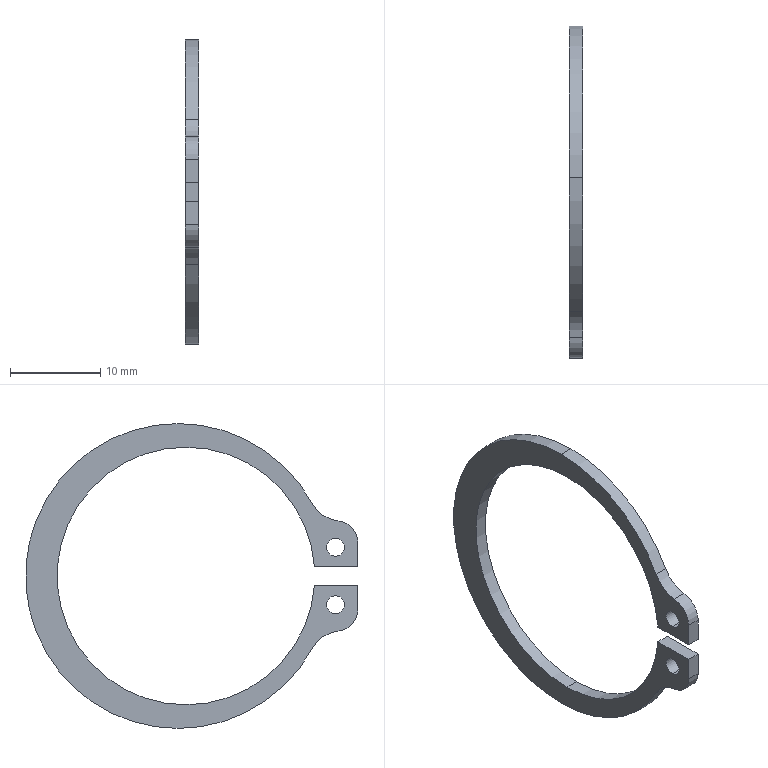Part | STEP file | 0229_005_STWN30 | 1 solid | 20 faces | box 1.5 x 36.9 x 33.85 mm | volume 424.063 mm3 | cylinder 14 | plane 6 | commonest cylinder face diameters 2 x4 28.6 x3 33.85 x3 5 x2 7.5 x2